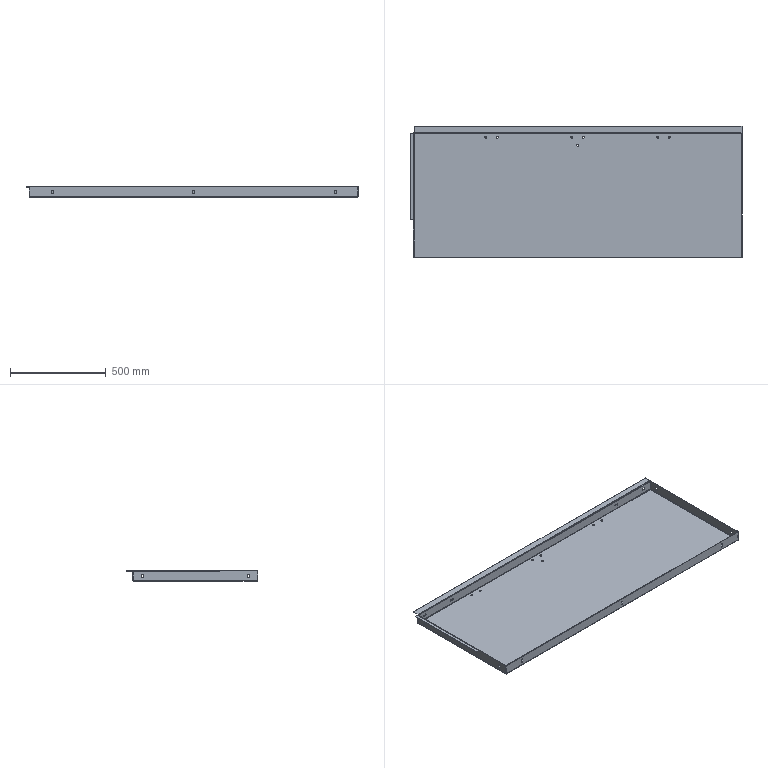Part | STEP file | SYL_0392D6J1SYL0380DJ100-608900 | 1 solid | 131 faces | box 1738 x 689 x 55 mm | volume 2865327 mm3 | cylinder 62 | plane 61 | spline 8 | commonest cylinder face diameters 10 x36 10.5 x12 4 x6 8 x6 9 x2